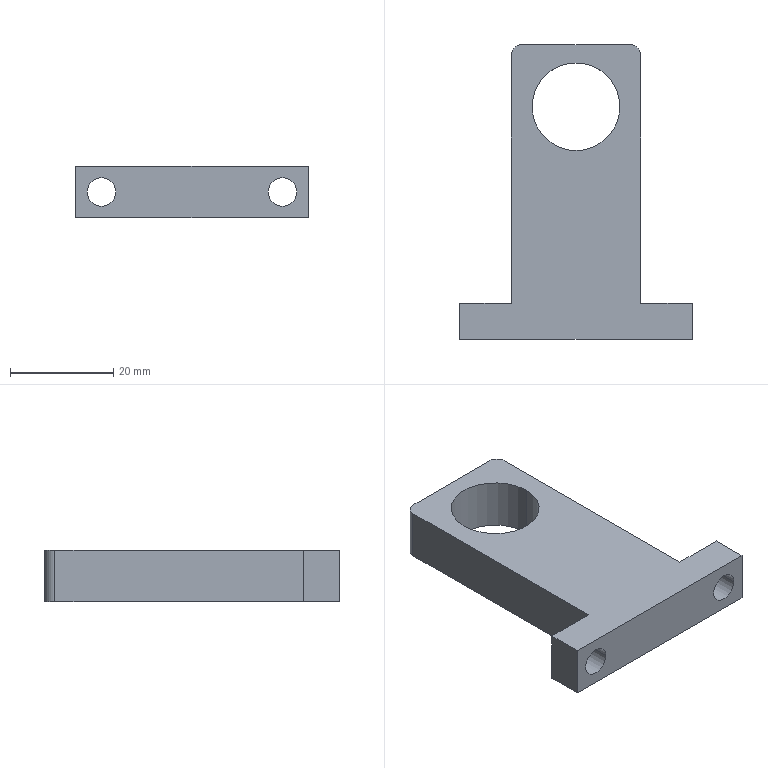Part | SolidWorks | features Extrusion 1, Fillet 1, ICE 1 | 1 solid | 18 faces | box 45 x 57 x 10 mm | volume 13030 mm3 | plane 10 | cylinder 8 | commonest cylinder face diameters 5.5 x4 4 x2 17 x2
STEP:
#1=CARTESIAN_POINT('',(-20.25,0.,0.));
#2=VERTEX_POINT('',#1);
#3=CARTESIAN_POINT('',(-14.75,0.,0.));
#4=VERTEX_POINT('',#3);
#5=CARTESIAN_POINT('',(-17.5,0.,0.));
#6=DIRECTION('',(0.,-1.,0.));
#7=DIRECTION('',(-1.,0.,0.));
#8=AXIS2_PLACEMENT_3D('',#5,#6,#7);
#9=CIRCLE('',#8,2.75);
#10=EDGE_CURVE('',#2,#4,#9,.T.);
#11=ORIENTED_EDGE('',*,*,#10,.T.);
#12=CARTESIAN_POINT('',(-14.75,7.,0.));
#13=VERTEX_POINT('',#12);
#14=CARTESIAN_POINT('',(-14.75,-0.001,0.));
#15=DIRECTION('',(0.,1.,0.));
#16=VECTOR('',#15,1000.);
#17=LINE('',#14,#16);
#18=EDGE_CURVE('',#4,#13,#17,.T.);
#19=ORIENTED_EDGE('',*,*,#18,.T.);
#20=CARTESIAN_POINT('',(-20.25,7.,0.));
#21=VERTEX_POINT('',#20);
#22=CARTESIAN_POINT('',(-17.5,7.,0.));
#23=DIRECTION('',(0.,1.,0.));
#24=DIRECTION('',(-1.,0.,0.));
#25=AXIS2_PLACEMENT_3D('',#22,#23,#24);
#26=CIRCLE('',#25,2.75);
#27=EDGE_CURVE('',#13,#21,#26,.T.);
#28=ORIENTED_EDGE('',*,*,#27,.T.);
#29=CARTESIAN_POINT('',(-20.25,-0.001,0.));
#30=DIRECTION('',(0.,1.,0.));
#31=VECTOR('',#30,1000.);
#32=LINE('',#29,#31);
#33=EDGE_CURVE('',#2,#21,#32,.T.);
#34=ORIENTED_EDGE('',*,*,#33,.F.);
#35=EDGE_LOOP('',(#11,#19,#28,#34));
#36=FACE_OUTER_BOUND('',#35,.T.);
#37=CARTESIAN_POINT('',(-17.5,-0.001,0.));
#38=DIRECTION('',(0.,1.,0.));
#39=DIRECTION('',(-1.,0.,0.));
#40=AXIS2_PLACEMENT_3D('',#37,#38,#39);
#41=CYLINDRICAL_SURFACE('',#40,2.75);
#42=ADVANCED_FACE('',(#36),#41,.F.);
#43=CARTESIAN_POINT('',(14.75,0.,0.));
#44=VERTEX_POINT('',#43);
#45=CARTESIAN_POINT('',(20.25,0.,0.));
#46=VERTEX_POINT('',#45);
#47=CARTESIAN_POINT('',(17.5,0.,0.));
#48=DIRECTION('',(0.,-1.,0.));
#49=DIRECTION('',(-1.,0.,0.));
#50=AXIS2_PLACEMENT_3D('',#47,#48,#49);
#51=CIRCLE('',#50,2.75);
#52=EDGE_CURVE('',#44,#46,#51,.T.);
#53=ORIENTED_EDGE('',*,*,#52,.T.);
#54=CARTESIAN_POINT('',(20.25,7.,0.));
#55=VERTEX_POINT('',#54);
#56=CARTESIAN_POINT('',(20.25,-0.001,0.));
#57=DIRECTION('',(0.,1.,0.));
#58=VECTOR('',#57,1000.);
#59=LINE('',#56,#58);
#60=EDGE_CURVE('',#46,#55,#59,.T.);
#61=ORIENTED_EDGE('',*,*,#60,.T.);
#62=CARTESIAN_POINT('',(14.75,7.,0.));
#63=VERTEX_POINT('',#62);
#64=CARTESIAN_POINT('',(17.5,7.,0.));
#65=DIRECTION('',(0.,1.,0.));
#66=DIRECTION('',(-1.,0.,0.));
#67=AXIS2_PLACEMENT_3D('',#64,#65,#66);
#68=CIRCLE('',#67,2.75);
#69=EDGE_CURVE('',#55,#63,#68,.T.);
#70=ORIENTED_EDGE('',*,*,#69,.T.);
#71=CARTESIAN_POINT('',(14.75,-0.001,0.));
#72=DIRECTION('',(0.,1.,0.));
#73=VECTOR('',#72,1000.);
#74=LINE('',#71,#73);
#75=EDGE_CURVE('',#44,#63,#74,.T.);
#76=ORIENTED_EDGE('',*,*,#75,.F.);
#77=EDGE_LOOP('',(#53,#61,#70,#76));
#78=FACE_OUTER_BOUND('',#77,.T.);
#79=CARTESIAN_POINT('',(17.5,-0.001,0.));
#80=DIRECTION('',(0.,1.,0.));
#81=DIRECTION('',(-1.,0.,0.));
#82=AXIS2_PLACEMENT_3D('',#79,#80,#81);
#83=CYLINDRICAL_SURFACE('',#82,2.75);
#84=ADVANCED_FACE('',(#78),#83,.F.);
#85=CARTESIAN_POINT('',(-8.5,45.,5.));
#86=VERTEX_POINT('',#85);
#87=CARTESIAN_POINT('',(8.5,45.,5.));
#88=VERTEX_POINT('',#87);
#89=CARTESIAN_POINT('',(0.,45.,5.));
#90=DIRECTION('',(0.,0.,1.));
#91=DIRECTION('',(1.,0.,0.));
#92=AXIS2_PLACEMENT_3D('',#89,#90,#91);
#93=CIRCLE('',#92,8.5);
#94=EDGE_CURVE('',#86,#88,#93,.T.);
#95=ORIENTED_EDGE('',*,*,#94,.T.);
#96=CARTESIAN_POINT('',(8.5,45.,-5.));
#97=VERTEX_POINT('',#96);
#98=CARTESIAN_POINT('',(8.5,45.,5.));
#99=DIRECTION('',(0.,0.,-1.));
#100=VECTOR('',#99,1000.);
#101=LINE('',#98,#100);
#102=EDGE_CURVE('',#88,#97,#101,.T.);
#103=ORIENTED_EDGE('',*,*,#102,.T.);
#104=CARTESIAN_POINT('',(-8.5,45.,-5.));
#105=VERTEX_POINT('',#104);
#106=CARTESIAN_POINT('',(0.,45.,-5.));
#107=DIRECTION('',(0.,0.,1.));
#108=DIRECTION('',(1.,0.,0.));
#109=AXIS2_PLACEMENT_3D('',#106,#107,#108);
#110=CIRCLE('',#109,8.5);
#111=EDGE_CURVE('',#105,#97,#110,.T.);
#112=ORIENTED_EDGE('',*,*,#111,.F.);
#113=CARTESIAN_POINT('',(-8.5,45.,5.));
#114=DIRECTION('',(0.,0.,-1.));
#115=VECTOR('',#114,1000.);
#116=LINE('',#113,#115);
#117=EDGE_CURVE('',#86,#105,#116,.T.);
#118=ORIENTED_EDGE('',*,*,#117,.F.);
#119=EDGE_LOOP('',(#95,#103,#112,#118));
#120=FACE_OUTER_BOUND('',#119,.T.);
#121=CARTESIAN_POINT('',(0.,45.,5.));
#122=DIRECTION('',(0.,0.,-1.));
#123=DIRECTION('',(-1.,0.,0.));
#124=AXIS2_PLACEMENT_3D('',#121,#122,#123);
#125=CYLINDRICAL_SURFACE('',#124,8.5);
#126=ADVANCED_FACE('',(#120),#125,.F.);
#127=CARTESIAN_POINT('',(10.5,57.,5.));
#128=VERTEX_POINT('',#127);
#129=CARTESIAN_POINT('',(-10.5,57.,5.));
#130=VERTEX_POINT('',#129);
#131=CARTESIAN_POINT('',(-12.5,57.,5.));
#132=DIRECTION('',(-1.,0.,0.));
#133=VECTOR('',#132,1000.);
#134=LINE('',#131,#133);
#135=EDGE_CURVE('',#128,#130,#134,.T.);
#136=ORIENTED_EDGE('',*,*,#135,.T.);
#137=CARTESIAN_POINT('',(-12.5,55.,5.));
#138=VERTEX_POINT('',#137);
#139=CARTESIAN_POINT('',(-10.5,55.,5.));
#140=DIRECTION('',(0.,0.,1.));
#141=DIRECTION('',(-1.,0.,0.));
#142=AXIS2_PLACEMENT_3D('',#139,#140,#141);
#143=CIRCLE('',#142,2.);
#144=EDGE_CURVE('',#130,#138,#143,.T.);
#145=ORIENTED_EDGE('',*,*,#144,.T.);
#146=CARTESIAN_POINT('',(-12.5,7.,5.));
#147=VERTEX_POINT('',#146);
#148=CARTESIAN_POINT('',(-12.5,7.,5.));
#149=DIRECTION('',(0.,-1.,0.));
#150=VECTOR('',#149,1000.);
#151=LINE('',#148,#150);
#152=EDGE_CURVE('',#138,#147,#151,.T.);
#153=ORIENTED_EDGE('',*,*,#152,.T.);
#154=CARTESIAN_POINT('',(-22.5,7.,5.));
#155=VERTEX_POINT('',#154);
#156=CARTESIAN_POINT('',(-22.5,7.,5.));
#157=DIRECTION('',(-1.,0.,0.));
#158=VECTOR('',#157,1000.);
#159=LINE('',#156,#158);
#160=EDGE_CURVE('',#147,#155,#159,.T.);
#161=ORIENTED_EDGE('',*,*,#160,.T.);
#162=CARTESIAN_POINT('',(-22.5,0.,5.));
#163=VERTEX_POINT('',#162);
#164=CARTESIAN_POINT('',(-22.5,0.,5.));
#165=DIRECTION('',(0.,-1.,0.));
#166=VECTOR('',#165,1000.);
#167=LINE('',#164,#166);
#168=EDGE_CURVE('',#155,#163,#167,.T.);
#169=ORIENTED_EDGE('',*,*,#168,.T.);
#170=CARTESIAN_POINT('',(22.5,0.,5.));
#171=VERTEX_POINT('',#170);
#172=CARTESIAN_POINT('',(22.5,0.,5.));
#173=DIRECTION('',(1.,0.,0.));
#174=VECTOR('',#173,1000.);
#175=LINE('',#172,#174);
#176=EDGE_CURVE('',#163,#171,#175,.T.);
#177=ORIENTED_EDGE('',*,*,#176,.T.);
#178=CARTESIAN_POINT('',(22.5,7.,5.));
#179=VERTEX_POINT('',#178);
#180=CARTESIAN_POINT('',(22.5,7.,5.));
#181=DIRECTION('',(0.,1.,0.));
#182=VECTOR('',#181,1000.);
#183=LINE('',#180,#182);
#184=EDGE_CURVE('',#171,#179,#183,.T.);
#185=ORIENTED_EDGE('',*,*,#184,.T.);
#186=CARTESIAN_POINT('',(12.5,7.,5.));
#187=VERTEX_POINT('',#186);
#188=CARTESIAN_POINT('',(12.5,7.,5.));
#189=DIRECTION('',(-1.,0.,0.));
#190=VECTOR('',#189,1000.);
#191=LINE('',#188,#190);
#192=EDGE_CURVE('',#179,#187,#191,.T.);
#193=ORIENTED_EDGE('',*,*,#192,.T.);
#194=CARTESIAN_POINT('',(12.5,55.,5.));
#195=VERTEX_POINT('',#194);
#196=CARTESIAN_POINT('',(12.5,57.,5.));
#197=DIRECTION('',(0.,1.,0.));
#198=VECTOR('',#197,1000.);
#199=LINE('',#196,#198);
#200=EDGE_CURVE('',#187,#195,#199,.T.);
#201=ORIENTED_EDGE('',*,*,#200,.T.);
#202=CARTESIAN_POINT('',(10.5,55.,5.));
#203=DIRECTION('',(0.,0.,1.));
#204=DIRECTION('',(-1.,0.,0.));
#205=AXIS2_PLACEMENT_3D('',#202,#203,#204);
#206=CIRCLE('',#205,2.);
#207=EDGE_CURVE('',#195,#128,#206,.T.);
#208=ORIENTED_EDGE('',*,*,#207,.T.);
#209=EDGE_LOOP('',(#136,#145,#153,#161,#169,#177,#185,#193,#201,#208));
#210=FACE_OUTER_BOUND('',#209,.T.);
#211=ORIENTED_EDGE('',*,*,#94,.F.);
#212=CARTESIAN_POINT('',(0.,45.,5.));
#213=DIRECTION('',(0.,0.,1.));
#214=DIRECTION('',(1.,0.,0.));
#215=AXIS2_PLACEMENT_3D('',#212,#213,#214);
#216=CIRCLE('',#215,8.5);
#217=EDGE_CURVE('',#88,#86,#216,.T.);
#218=ORIENTED_EDGE('',*,*,#217,.F.);
#219=EDGE_LOOP('',(#211,#218));
#220=FACE_BOUND('',#219,.T.);
#221=CARTESIAN_POINT('',(0.,0.,5.));
#222=DIRECTION('',(0.,0.,-1.));
#223=DIRECTION('',(-1.,0.,0.));
#224=AXIS2_PLACEMENT_3D('',#221,#222,#223);
#225=PLANE('',#224);
#226=ADVANCED_FACE('',(#210,#220),#225,.F.);
#227=CARTESIAN_POINT('',(-12.5,55.,-5.));
#228=VERTEX_POINT('',#227);
#229=CARTESIAN_POINT('',(-12.5,7.,-5.));
#230=VERTEX_POINT('',#229);
#231=CARTESIAN_POINT('',(-12.5,7.,-5.));
#232=DIRECTION('',(0.,-1.,0.));
#233=VECTOR('',#232,1000.);
#234=LINE('',#231,#233);
#235=EDGE_CURVE('',#228,#230,#234,.T.);
#236=ORIENTED_EDGE('',*,*,#235,.F.);
#237=CARTESIAN_POINT('',(-10.5,57.,-5.));
#238=VERTEX_POINT('',#237);
#239=CARTESIAN_POINT('',(-10.5,55.,-5.));
#240=DIRECTION('',(0.,0.,-1.));
#241=DIRECTION('',(-1.,0.,0.));
#242=AXIS2_PLACEMENT_3D('',#239,#240,#241);
#243=CIRCLE('',#242,2.);
#244=EDGE_CURVE('',#228,#238,#243,.T.);
#245=ORIENTED_EDGE('',*,*,#244,.T.);
#246=CARTESIAN_POINT('',(10.5,57.,-5.));
#247=VERTEX_POINT('',#246);
#248=CARTESIAN_POINT('',(-12.5,57.,-5.));
#249=DIRECTION('',(-1.,0.,0.));
#250=VECTOR('',#249,1000.);
#251=LINE('',#248,#250);
#252=EDGE_CURVE('',#247,#238,#251,.T.);
#253=ORIENTED_EDGE('',*,*,#252,.F.);
#254=CARTESIAN_POINT('',(12.5,55.,-5.));
#255=VERTEX_POINT('',#254);
#256=CARTESIAN_POINT('',(10.5,55.,-5.));
#257=DIRECTION('',(0.,0.,-1.));
#258=DIRECTION('',(-1.,0.,0.));
#259=AXIS2_PLACEMENT_3D('',#256,#257,#258);
#260=CIRCLE('',#259,2.);
#261=EDGE_CURVE('',#247,#255,#260,.T.);
#262=ORIENTED_EDGE('',*,*,#261,.T.);
#263=CARTESIAN_POINT('',(12.5,7.,-5.));
#264=VERTEX_POINT('',#263);
#265=CARTESIAN_POINT('',(12.5,57.,-5.));
#266=DIRECTION('',(0.,1.,0.));
#267=VECTOR('',#266,1000.);
#268=LINE('',#265,#267);
#269=EDGE_CURVE('',#264,#255,#268,.T.);
#270=ORIENTED_EDGE('',*,*,#269,.F.);
#271=CARTESIAN_POINT('',(22.5,7.,-5.));
#272=VERTEX_POINT('',#271);
#273=CARTESIAN_POINT('',(12.5,7.,-5.));
#274=DIRECTION('',(-1.,0.,0.));
#275=VECTOR('',#274,1000.);
#276=LINE('',#273,#275);
#277=EDGE_CURVE('',#272,#264,#276,.T.);
#278=ORIENTED_EDGE('',*,*,#277,.F.);
#279=CARTESIAN_POINT('',(22.5,0.,-5.));
#280=VERTEX_POINT('',#279);
#281=CARTESIAN_POINT('',(22.5,7.,-5.));
#282=DIRECTION('',(0.,1.,0.));
#283=VECTOR('',#282,1000.);
#284=LINE('',#281,#283);
#285=EDGE_CURVE('',#280,#272,#284,.T.);
#286=ORIENTED_EDGE('',*,*,#285,.F.);
#287=CARTESIAN_POINT('',(-22.5,0.,-5.));
#288=VERTEX_POINT('',#287);
#289=CARTESIAN_POINT('',(0.,0.,-5.));
#290=DIRECTION('',(1.,0.,0.));
#291=VECTOR('',#290,1000.);
#292=LINE('',#289,#291);
#293=EDGE_CURVE('',#288,#280,#292,.T.);
#294=ORIENTED_EDGE('',*,*,#293,.F.);
#295=CARTESIAN_POINT('',(-22.5,7.,-5.));
#296=VERTEX_POINT('',#295);
#297=CARTESIAN_POINT('',(-22.5,0.,-5.));
#298=DIRECTION('',(0.,-1.,0.));
#299=VECTOR('',#298,1000.);
#300=LINE('',#297,#299);
#301=EDGE_CURVE('',#296,#288,#300,.T.);
#302=ORIENTED_EDGE('',*,*,#301,.F.);
#303=CARTESIAN_POINT('',(-22.5,7.,-5.));
#304=DIRECTION('',(-1.,0.,0.));
#305=VECTOR('',#304,1000.);
#306=LINE('',#303,#305);
#307=EDGE_CURVE('',#230,#296,#306,.T.);
#308=ORIENTED_EDGE('',*,*,#307,.F.);
#309=EDGE_LOOP('',(#236,#245,#253,#262,#270,#278,#286,#294,#302,#308));
#310=FACE_OUTER_BOUND('',#309,.T.);
#311=ORIENTED_EDGE('',*,*,#111,.T.);
#312=CARTESIAN_POINT('',(0.,45.,-5.));
#313=DIRECTION('',(0.,0.,1.));
#314=DIRECTION('',(1.,0.,0.));
#315=AXIS2_PLACEMENT_3D('',#312,#313,#314);
#316=CIRCLE('',#315,8.5);
#317=EDGE_CURVE('',#97,#105,#316,.T.);
#318=ORIENTED_EDGE('',*,*,#317,.T.);
#319=EDGE_LOOP('',(#311,#318));
#320=FACE_BOUND('',#319,.T.);
#321=CARTESIAN_POINT('',(0.,0.,-5.));
#322=DIRECTION('',(0.,0.,-1.));
#323=DIRECTION('',(-1.,0.,0.));
#324=AXIS2_PLACEMENT_3D('',#321,#322,#323);
#325=PLANE('',#324);
#326=ADVANCED_FACE('',(#310,#320),#325,.T.);
#327=ORIENTED_EDGE('',*,*,#285,.T.);
#328=CARTESIAN_POINT('',(22.5,7.,5.));
#329=DIRECTION('',(0.,0.,-1.));
#330=VECTOR('',#329,1000.);
#331=LINE('',#328,#330);
#332=EDGE_CURVE('',#179,#272,#331,.T.);
#333=ORIENTED_EDGE('',*,*,#332,.F.);
#334=ORIENTED_EDGE('',*,*,#184,.F.);
#335=CARTESIAN_POINT('',(22.5,0.,5.));
#336=DIRECTION('',(0.,0.,-1.));
#337=VECTOR('',#336,1000.);
#338=LINE('',#335,#337);
#339=EDGE_CURVE('',#171,#280,#338,.T.);
#340=ORIENTED_EDGE('',*,*,#339,.T.);
#341=EDGE_LOOP('',(#327,#333,#334,#340));
#342=FACE_OUTER_BOUND('',#341,.T.);
#343=CARTESIAN_POINT('',(22.5,7.,5.));
#344=DIRECTION('',(-1.,0.,0.));
#345=DIRECTION('',(0.,-1.,0.));
#346=AXIS2_PLACEMENT_3D('',#343,#344,#345);
#347=PLANE('',#346);
#348=ADVANCED_FACE('',(#342),#347,.F.);
#349=CARTESIAN_POINT('',(17.5,7.,0.));
#350=DIRECTION('',(0.,1.,0.));
#351=DIRECTION('',(-1.,0.,0.));
#352=AXIS2_PLACEMENT_3D('',#349,#350,#351);
#353=CIRCLE('',#352,2.75);
#354=EDGE_CURVE('',#63,#55,#353,.T.);
#355=ORIENTED_EDGE('',*,*,#354,.F.);
#356=ORIENTED_EDGE('',*,*,#69,.F.);
#357=EDGE_LOOP('',(#355,#356));
#358=FACE_BOUND('',#357,.T.);
#359=ORIENTED_EDGE('',*,*,#277,.T.);
#360=CARTESIAN_POINT('',(12.5,7.,5.));
#361=DIRECTION('',(0.,0.,-1.));
#362=VECTOR('',#361,1000.);
#363=LINE('',#360,#362);
#364=EDGE_CURVE('',#187,#264,#363,.T.);
#365=ORIENTED_EDGE('',*,*,#364,.F.);
#366=ORIENTED_EDGE('',*,*,#192,.F.);
#367=ORIENTED_EDGE('',*,*,#332,.T.);
#368=EDGE_LOOP('',(#359,#365,#366,#367));
#369=FACE_OUTER_BOUND('',#368,.T.);
#370=CARTESIAN_POINT('',(12.5,7.,5.));
#371=DIRECTION('',(0.,-1.,0.));
#372=DIRECTION('',(1.,0.,0.));
#373=AXIS2_PLACEMENT_3D('',#370,#371,#372);
#374=PLANE('',#373);
#375=ADVANCED_FACE('',(#358,#369),#374,.F.);
#376=ORIENTED_EDGE('',*,*,#269,.T.);
#377=CARTESIAN_POINT('',(12.5,55.,5.));
#378=DIRECTION('',(0.,0.,1.));
#379=VECTOR('',#378,1000.);
#380=LINE('',#377,#379);
#381=EDGE_CURVE('',#255,#195,#380,.T.);
#382=ORIENTED_EDGE('',*,*,#381,.T.);
#383=ORIENTED_EDGE('',*,*,#200,.F.);
#384=ORIENTED_EDGE('',*,*,#364,.T.);
#385=EDGE_LOOP('',(#376,#382,#383,#384));
#386=FACE_OUTER_BOUND('',#385,.T.);
#387=CARTESIAN_POINT('',(12.5,57.,5.));
#388=DIRECTION('',(-1.,0.,0.));
#389=DIRECTION('',(0.,-1.,0.));
#390=AXIS2_PLACEMENT_3D('',#387,#388,#389);
#391=PLANE('',#390);
#392=ADVANCED_FACE('',(#386),#391,.F.);
#393=ORIENTED_EDGE('',*,*,#252,.T.);
#394=CARTESIAN_POINT('',(-10.5,57.,5.));
#395=DIRECTION('',(0.,0.,1.));
#396=VECTOR('',#395,1000.);
#397=LINE('',#394,#396);
#398=EDGE_CURVE('',#238,#130,#397,.T.);
#399=ORIENTED_EDGE('',*,*,#398,.T.);
#400=ORIENTED_EDGE('',*,*,#135,.F.);
#401=CARTESIAN_POINT('',(10.5,57.,5.));
#402=DIRECTION('',(0.,0.,-1.));
#403=VECTOR('',#402,1000.);
#404=LINE('',#401,#403);
#405=EDGE_CURVE('',#128,#247,#404,.T.);
#406=ORIENTED_EDGE('',*,*,#405,.T.);
#407=EDGE_LOOP('',(#393,#399,#400,#406));
#408=FACE_OUTER_BOUND('',#407,.T.);
#409=CARTESIAN_POINT('',(-12.5,57.,5.));
#410=DIRECTION('',(0.,-1.,0.));
#411=DIRECTION('',(0.,0.,-1.));
#412=AXIS2_PLACEMENT_3D('',#409,#410,#411);
#413=PLANE('',#412);
#414=ADVANCED_FACE('',(#408),#413,.F.);
#415=ORIENTED_EDGE('',*,*,#152,.F.);
#416=CARTESIAN_POINT('',(-12.5,55.,5.));
#417=DIRECTION('',(0.,0.,-1.));
#418=VECTOR('',#417,1000.);
#419=LINE('',#416,#418);
#420=EDGE_CURVE('',#138,#228,#419,.T.);
#421=ORIENTED_EDGE('',*,*,#420,.T.);
#422=ORIENTED_EDGE('',*,*,#235,.T.);
#423=CARTESIAN_POINT('',(-12.5,7.,5.));
#424=DIRECTION('',(0.,0.,-1.));
#425=VECTOR('',#424,1000.);
#426=LINE('',#423,#425);
#427=EDGE_CURVE('',#147,#230,#426,.T.);
#428=ORIENTED_EDGE('',*,*,#427,.F.);
#429=EDGE_LOOP('',(#415,#421,#422,#428));
#430=FACE_OUTER_BOUND('',#429,.T.);
#431=CARTESIAN_POINT('',(-12.5,7.,5.));
#432=DIRECTION('',(1.,0.,0.));
#433=DIRECTION('',(0.,0.,-1.));
#434=AXIS2_PLACEMENT_3D('',#431,#432,#433);
#435=PLANE('',#434);
#436=ADVANCED_FACE('',(#430),#435,.F.);
#437=CARTESIAN_POINT('',(-17.5,7.,0.));
#438=DIRECTION('',(0.,1.,0.));
#439=DIRECTION('',(-1.,0.,0.));
#440=AXIS2_PLACEMENT_3D('',#437,#438,#439);
#441=CIRCLE('',#440,2.75);
#442=EDGE_CURVE('',#21,#13,#441,.T.);
#443=ORIENTED_EDGE('',*,*,#442,.F.);
#444=ORIENTED_EDGE('',*,*,#27,.F.);
#445=EDGE_LOOP('',(#443,#444));
#446=FACE_BOUND('',#445,.T.);
#447=ORIENTED_EDGE('',*,*,#307,.T.);
#448=CARTESIAN_POINT('',(-22.5,7.,5.));
#449=DIRECTION('',(0.,0.,-1.));
#450=VECTOR('',#449,1000.);
#451=LINE('',#448,#450);
#452=EDGE_CURVE('',#155,#296,#451,.T.);
#453=ORIENTED_EDGE('',*,*,#452,.F.);
#454=ORIENTED_EDGE('',*,*,#160,.F.);
#455=ORIENTED_EDGE('',*,*,#427,.T.);
#456=EDGE_LOOP('',(#447,#453,#454,#455));
#457=FACE_OUTER_BOUND('',#456,.T.);
#458=CARTESIAN_POINT('',(-22.5,7.,5.));
#459=DIRECTION('',(0.,-1.,0.));
#460=DIRECTION('',(1.,0.,0.));
#461=AXIS2_PLACEMENT_3D('',#458,#459,#460);
#462=PLANE('',#461);
#463=ADVANCED_FACE('',(#446,#457),#462,.F.);
#464=ORIENTED_EDGE('',*,*,#301,.T.);
#465=CARTESIAN_POINT('',(-22.5,0.,5.));
#466=DIRECTION('',(0.,0.,-1.));
#467=VECTOR('',#466,1000.);
#468=LINE('',#465,#467);
#469=EDGE_CURVE('',#163,#288,#468,.T.);
#470=ORIENTED_EDGE('',*,*,#469,.F.);
#471=ORIENTED_EDGE('',*,*,#168,.F.);
#472=ORIENTED_EDGE('',*,*,#452,.T.);
#473=EDGE_LOOP('',(#464,#470,#471,#472));
#474=FACE_OUTER_BOUND('',#473,.T.);
#475=CARTESIAN_POINT('',(-22.5,0.,5.));
#476=DIRECTION('',(1.,0.,0.));
#477=DIRECTION('',(0.,0.,-1.));
#478=AXIS2_PLACEMENT_3D('',#475,#476,#477);
#479=PLANE('',#478);
#480=ADVANCED_FACE('',(#474),#479,.F.);
#481=ORIENTED_EDGE('',*,*,#10,.F.);
#482=CARTESIAN_POINT('',(-17.5,0.,0.));
#483=DIRECTION('',(0.,-1.,0.));
#484=DIRECTION('',(-1.,0.,0.));
#485=AXIS2_PLACEMENT_3D('',#482,#483,#484);
#486=CIRCLE('',#485,2.75);
#487=EDGE_CURVE('',#4,#2,#486,.T.);
#488=ORIENTED_EDGE('',*,*,#487,.F.);
#489=EDGE_LOOP('',(#481,#488));
#490=FACE_BOUND('',#489,.T.);
#491=ORIENTED_EDGE('',*,*,#52,.F.);
#492=CARTESIAN_POINT('',(17.5,0.,0.));
#493=DIRECTION('',(0.,-1.,0.));
#494=DIRECTION('',(-1.,0.,0.));
#495=AXIS2_PLACEMENT_3D('',#492,#493,#494);
#496=CIRCLE('',#495,2.75);
#497=EDGE_CURVE('',#46,#44,#496,.T.);
#498=ORIENTED_EDGE('',*,*,#497,.F.);
#499=EDGE_LOOP('',(#491,#498));
#500=FACE_BOUND('',#499,.T.);
#501=ORIENTED_EDGE('',*,*,#293,.T.);
#502=ORIENTED_EDGE('',*,*,#339,.F.);
#503=ORIENTED_EDGE('',*,*,#176,.F.);
#504=ORIENTED_EDGE('',*,*,#469,.T.);
#505=EDGE_LOOP('',(#501,#502,#503,#504));
#506=FACE_OUTER_BOUND('',#505,.T.);
#507=CARTESIAN_POINT('',(0.,0.,5.));
#508=DIRECTION('',(0.,1.,0.));
#509=DIRECTION('',(-1.,0.,0.));
#510=AXIS2_PLACEMENT_3D('',#507,#508,#509);
#511=PLANE('',#510);
#512=ADVANCED_FACE('',(#490,#500,#506),#511,.F.);
#513=ORIENTED_EDGE('',*,*,#102,.F.);
#514=ORIENTED_EDGE('',*,*,#217,.T.);
#515=ORIENTED_EDGE('',*,*,#117,.T.);
#516=ORIENTED_EDGE('',*,*,#317,.F.);
#517=EDGE_LOOP('',(#513,#514,#515,#516));
#518=FACE_OUTER_BOUND('',#517,.T.);
#519=CARTESIAN_POINT('',(0.,45.,5.));
#520=DIRECTION('',(0.,0.,-1.));
#521=DIRECTION('',(-1.,0.,0.));
#522=AXIS2_PLACEMENT_3D('',#519,#520,#521);
#523=CYLINDRICAL_SURFACE('',#522,8.5);
#524=ADVANCED_FACE('',(#518),#523,.F.);
#525=ORIENTED_EDGE('',*,*,#144,.F.);
#526=ORIENTED_EDGE('',*,*,#398,.F.);
#527=ORIENTED_EDGE('',*,*,#244,.F.);
#528=ORIENTED_EDGE('',*,*,#420,.F.);
#529=EDGE_LOOP('',(#525,#526,#527,#528));
#530=FACE_OUTER_BOUND('',#529,.T.);
#531=CARTESIAN_POINT('',(-10.5,55.,5.));
#532=DIRECTION('',(0.,0.,-1.));
#533=DIRECTION('',(-1.,0.,0.));
#534=AXIS2_PLACEMENT_3D('',#531,#532,#533);
#535=CYLINDRICAL_SURFACE('',#534,2.);
#536=ADVANCED_FACE('',(#530),#535,.T.);
#537=ORIENTED_EDGE('',*,*,#207,.F.);
#538=ORIENTED_EDGE('',*,*,#381,.F.);
#539=ORIENTED_EDGE('',*,*,#261,.F.);
#540=ORIENTED_EDGE('',*,*,#405,.F.);
#541=EDGE_LOOP('',(#537,#538,#539,#540));
#542=FACE_OUTER_BOUND('',#541,.T.);
#543=CARTESIAN_POINT('',(10.5,55.,5.));
#544=DIRECTION('',(0.,0.,-1.));
#545=DIRECTION('',(-1.,0.,0.));
#546=AXIS2_PLACEMENT_3D('',#543,#544,#545);
#547=CYLINDRICAL_SURFACE('',#546,2.);
#548=ADVANCED_FACE('',(#542),#547,.T.);
#549=ORIENTED_EDGE('',*,*,#60,.F.);
#550=ORIENTED_EDGE('',*,*,#497,.T.);
#551=ORIENTED_EDGE('',*,*,#75,.T.);
#552=ORIENTED_EDGE('',*,*,#354,.T.);
#553=EDGE_LOOP('',(#549,#550,#551,#552));
#554=FACE_OUTER_BOUND('',#553,.T.);
#555=CARTESIAN_POINT('',(17.5,-0.001,0.));
#556=DIRECTION('',(0.,1.,0.));
#557=DIRECTION('',(-1.,0.,0.));
#558=AXIS2_PLACEMENT_3D('',#555,#556,#557);
#559=CYLINDRICAL_SURFACE('',#558,2.75);
#560=ADVANCED_FACE('',(#554),#559,.F.);
#561=ORIENTED_EDGE('',*,*,#18,.F.);
#562=ORIENTED_EDGE('',*,*,#487,.T.);
#563=ORIENTED_EDGE('',*,*,#33,.T.);
#564=ORIENTED_EDGE('',*,*,#442,.T.);
#565=EDGE_LOOP('',(#561,#562,#563,#564));
#566=FACE_OUTER_BOUND('',#565,.T.);
#567=CARTESIAN_POINT('',(-17.5,-0.001,0.));
#568=DIRECTION('',(0.,1.,0.));
#569=DIRECTION('',(-1.,0.,0.));
#570=AXIS2_PLACEMENT_3D('',#567,#568,#569);
#571=CYLINDRICAL_SURFACE('',#570,2.75);
#572=ADVANCED_FACE('',(#566),#571,.F.);
#573=CLOSED_SHELL('',(#42,#84,#126,#226,#326,#348,#375,#392,#414,#436,#463,#480,#512,#524,#536,#548,#560,#572));
#574=MANIFOLD_SOLID_BREP('',#573);
#575=CARTESIAN_POINT('',(0.,0.,0.));
#576=DIRECTION('',(0.,0.,1.));
#577=DIRECTION('',(1.,0.,0.));
#578=AXIS2_PLACEMENT_3D('',#575,#576,#577);
#579=(LENGTH_UNIT()NAMED_UNIT(*)SI_UNIT(.MILLI.,.METRE.));
#580=UNCERTAINTY_MEASURE_WITH_UNIT(LENGTH_MEASURE(0.00001),#579,'','');
#581=(NAMED_UNIT(*)PLANE_ANGLE_UNIT()SI_UNIT($,.RADIAN.));
#582=(NAMED_UNIT(*)SI_UNIT($,.STERADIAN.)SOLID_ANGLE_UNIT());
#583=(GEOMETRIC_REPRESENTATION_CONTEXT(3)GLOBAL_UNCERTAINTY_ASSIGNED_CONTEXT((#580))GLOBAL_UNIT_ASSIGNED_CONTEXT((#579,#581,#582))REPRESENTATION_CONTEXT('',''));
#584=ADVANCED_BREP_SHAPE_REPRESENTATION('',(#574,#578),#583);